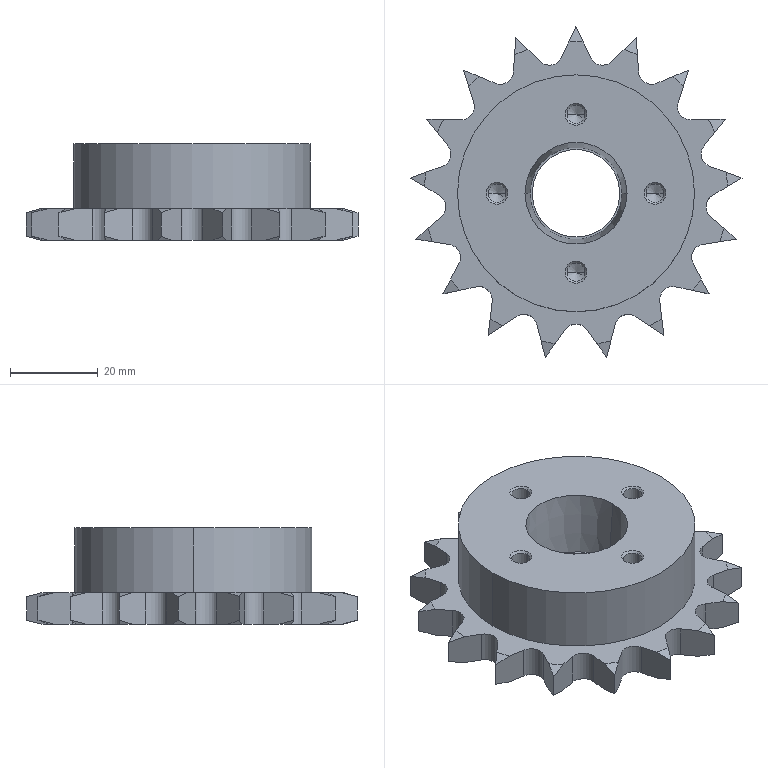Part | STEP file | LFSP40B17_20_Asp | 1 solid | 124 faces | box 75.676 x 75.353 x 22 mm | volume 49189 mm3 | cone 52 | plane 38 | cylinder 34 | commonest cylinder face diameters 6 x22 4.134 x8 20 x2 54 x2